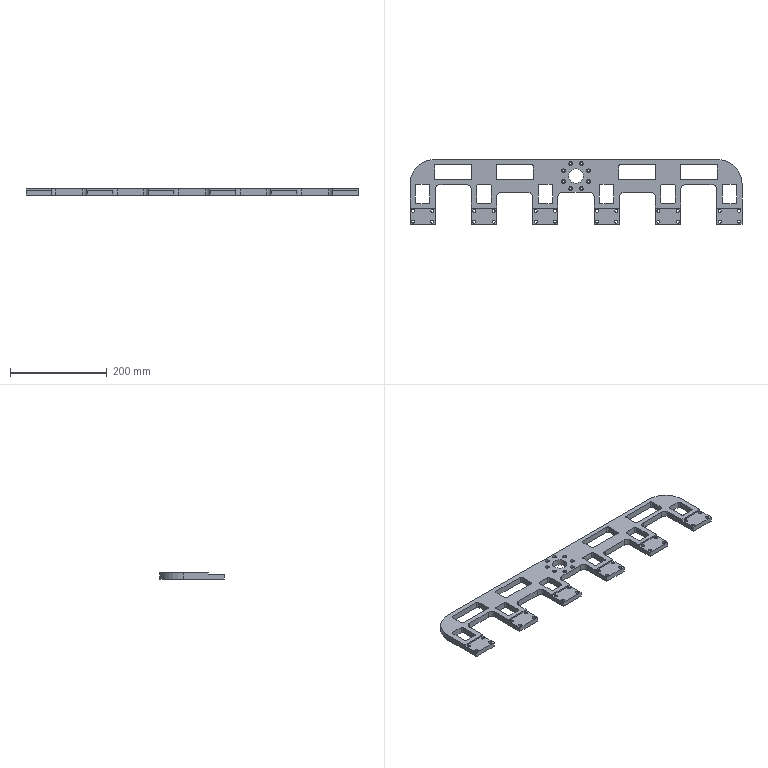Part | 1 solid | 179 faces | box 687 x 134 x 13 mm | volume 560254 mm3 | cylinder 93 | plane 86 | commonest cylinder face diameters 6 x40 6.5 x24 20 x10 4.5 x8 8 x8 100 x2